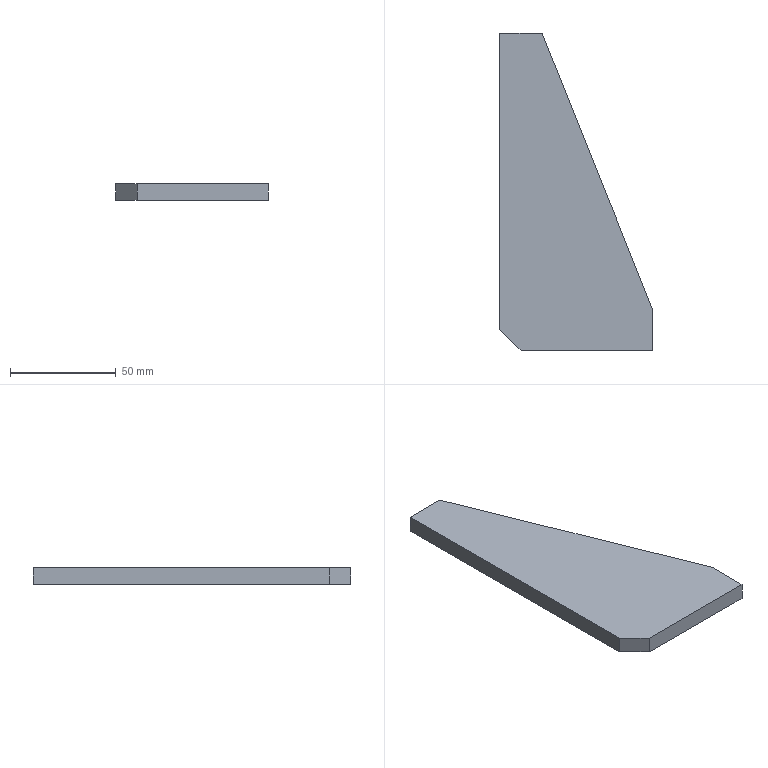Part | STEP file | 运输筋Plate 1 | 1 solid | 8 faces | box 72 x 150 x 8 mm | volume 58960 mm3 | plane 8
STEP:
#1=CARTESIAN_POINT('',(0.,0.,0.));
#2=DIRECTION('',(0.,0.,1.));
#3=DIRECTION('',(1.,0.,0.));
#4=AXIS2_PLACEMENT_3D('',#1,#2,#3);
#5=CARTESIAN_POINT('',(72.,0.,-4.));
#6=VERTEX_POINT('',#5);
#7=CARTESIAN_POINT('',(72.,20.,-4.));
#8=VERTEX_POINT('',#7);
#9=CARTESIAN_POINT('',(72.,0.,-4.));
#10=DIRECTION('',(0.,1.,0.));
#11=VECTOR('',#10,1.);
#12=LINE('',#9,#11);
#13=CARTESIAN_POINT('',(72.,0.,4.));
#14=DIRECTION('',(-1.,0.,0.));
#15=DIRECTION('',(0.,0.,1.));
#16=AXIS2_PLACEMENT_3D('',#13,#14,#15);
#17=PLANE('',#16);
#18=CARTESIAN_POINT('',(-8.,0.));
#19=DIRECTION('',(0.,1.));
#20=VECTOR('',#19,1.);
#21=LINE('',#18,#20);
#22=(GEOMETRIC_REPRESENTATION_CONTEXT(2)PARAMETRIC_REPRESENTATION_CONTEXT()REPRESENTATION_CONTEXT('',''));
#23=DEFINITIONAL_REPRESENTATION('',(#21),#22);
#24=PCURVE('',#17,#23);
#25=CARTESIAN_POINT('',(0.,0.,-4.));
#26=DIRECTION('',(0.,0.,1.));
#27=DIRECTION('',(1.,0.,0.));
#28=AXIS2_PLACEMENT_3D('',#25,#26,#27);
#29=PLANE('',#28);
#30=CARTESIAN_POINT('',(72.,0.));
#31=DIRECTION('',(0.,1.));
#32=VECTOR('',#31,1.);
#33=LINE('',#30,#32);
#34=(GEOMETRIC_REPRESENTATION_CONTEXT(2)PARAMETRIC_REPRESENTATION_CONTEXT()REPRESENTATION_CONTEXT('',''));
#35=DEFINITIONAL_REPRESENTATION('',(#33),#34);
#36=PCURVE('',#29,#35);
#37=SURFACE_CURVE('',#12,(#24,#36),.PCURVE_S1.);
#38=EDGE_CURVE('',#6,#8,#37,.T.);
#39=ORIENTED_EDGE('',*,*,#38,.T.);
#40=CARTESIAN_POINT('',(72.,20.,4.));
#41=VERTEX_POINT('',#40);
#42=CARTESIAN_POINT('',(72.,20.,4.));
#43=DIRECTION('',(0.,0.,-1.));
#44=VECTOR('',#43,1.);
#45=LINE('',#42,#44);
#46=CARTESIAN_POINT('',(0.,20.));
#47=DIRECTION('',(-1.,0.));
#48=VECTOR('',#47,1.);
#49=LINE('',#46,#48);
#50=(GEOMETRIC_REPRESENTATION_CONTEXT(2)PARAMETRIC_REPRESENTATION_CONTEXT()REPRESENTATION_CONTEXT('',''));
#51=DEFINITIONAL_REPRESENTATION('',(#49),#50);
#52=PCURVE('',#17,#51);
#53=CARTESIAN_POINT('',(72.,20.,4.));
#54=DIRECTION('',(-0.9285,-0.3714,0.));
#55=DIRECTION('',(0.3714,-0.9285,0.));
#56=AXIS2_PLACEMENT_3D('',#53,#54,#55);
#57=PLANE('',#56);
#58=CARTESIAN_POINT('',(0.,0.));
#59=DIRECTION('',(0.,-1.));
#60=VECTOR('',#59,1.);
#61=LINE('',#58,#60);
#62=(GEOMETRIC_REPRESENTATION_CONTEXT(2)PARAMETRIC_REPRESENTATION_CONTEXT()REPRESENTATION_CONTEXT('',''));
#63=DEFINITIONAL_REPRESENTATION('',(#61),#62);
#64=PCURVE('',#57,#63);
#65=SURFACE_CURVE('',#45,(#52,#64),.PCURVE_S1.);
#66=EDGE_CURVE('',#41,#8,#65,.T.);
#67=ORIENTED_EDGE('',*,*,#66,.F.);
#68=CARTESIAN_POINT('',(72.,0.,4.));
#69=VERTEX_POINT('',#68);
#70=CARTESIAN_POINT('',(72.,0.,4.));
#71=DIRECTION('',(0.,1.,0.));
#72=VECTOR('',#71,1.);
#73=LINE('',#70,#72);
#74=CARTESIAN_POINT('',(0.,0.));
#75=DIRECTION('',(0.,1.));
#76=VECTOR('',#75,1.);
#77=LINE('',#74,#76);
#78=(GEOMETRIC_REPRESENTATION_CONTEXT(2)PARAMETRIC_REPRESENTATION_CONTEXT()REPRESENTATION_CONTEXT('',''));
#79=DEFINITIONAL_REPRESENTATION('',(#77),#78);
#80=PCURVE('',#17,#79);
#81=CARTESIAN_POINT('',(0.,0.,4.));
#82=DIRECTION('',(0.,0.,1.));
#83=DIRECTION('',(1.,0.,0.));
#84=AXIS2_PLACEMENT_3D('',#81,#82,#83);
#85=PLANE('',#84);
#86=CARTESIAN_POINT('',(72.,0.));
#87=DIRECTION('',(0.,1.));
#88=VECTOR('',#87,1.);
#89=LINE('',#86,#88);
#90=(GEOMETRIC_REPRESENTATION_CONTEXT(2)PARAMETRIC_REPRESENTATION_CONTEXT()REPRESENTATION_CONTEXT('',''));
#91=DEFINITIONAL_REPRESENTATION('',(#89),#90);
#92=PCURVE('',#85,#91);
#93=SURFACE_CURVE('',#73,(#80,#92),.PCURVE_S1.);
#94=EDGE_CURVE('',#69,#41,#93,.T.);
#95=ORIENTED_EDGE('',*,*,#94,.F.);
#96=CARTESIAN_POINT('',(72.,0.,4.));
#97=DIRECTION('',(0.,0.,-1.));
#98=VECTOR('',#97,1.);
#99=LINE('',#96,#98);
#100=CARTESIAN_POINT('',(0.,0.));
#101=DIRECTION('',(-1.,0.));
#102=VECTOR('',#101,1.);
#103=LINE('',#100,#102);
#104=(GEOMETRIC_REPRESENTATION_CONTEXT(2)PARAMETRIC_REPRESENTATION_CONTEXT()REPRESENTATION_CONTEXT('',''));
#105=DEFINITIONAL_REPRESENTATION('',(#103),#104);
#106=PCURVE('',#17,#105);
#107=CARTESIAN_POINT('',(0.,0.,4.));
#108=DIRECTION('',(0.,1.,0.));
#109=DIRECTION('',(0.,0.,1.));
#110=AXIS2_PLACEMENT_3D('',#107,#108,#109);
#111=PLANE('',#110);
#112=CARTESIAN_POINT('',(0.,72.));
#113=DIRECTION('',(-1.,0.));
#114=VECTOR('',#113,1.);
#115=LINE('',#112,#114);
#116=(GEOMETRIC_REPRESENTATION_CONTEXT(2)PARAMETRIC_REPRESENTATION_CONTEXT()REPRESENTATION_CONTEXT('',''));
#117=DEFINITIONAL_REPRESENTATION('',(#115),#116);
#118=PCURVE('',#111,#117);
#119=SURFACE_CURVE('',#99,(#106,#118),.PCURVE_S1.);
#120=EDGE_CURVE('',#69,#6,#119,.T.);
#121=ORIENTED_EDGE('',*,*,#120,.T.);
#122=EDGE_LOOP('',(#39,#67,#95,#121));
#123=FACE_BOUND('',#122,.T.);
#124=ADVANCED_FACE('',(#123),#17,.F.);
#125=CARTESIAN_POINT('',(20.,150.,-4.));
#126=VERTEX_POINT('',#125);
#127=CARTESIAN_POINT('',(72.,20.,-4.));
#128=DIRECTION('',(-0.3714,0.9285,0.));
#129=VECTOR('',#128,1.);
#130=LINE('',#127,#129);
#131=CARTESIAN_POINT('',(0.,-8.));
#132=DIRECTION('',(-1.,0.));
#133=VECTOR('',#132,1.);
#134=LINE('',#131,#133);
#135=(GEOMETRIC_REPRESENTATION_CONTEXT(2)PARAMETRIC_REPRESENTATION_CONTEXT()REPRESENTATION_CONTEXT('',''));
#136=DEFINITIONAL_REPRESENTATION('',(#134),#135);
#137=PCURVE('',#57,#136);
#138=CARTESIAN_POINT('',(72.,20.));
#139=DIRECTION('',(-0.3714,0.9285));
#140=VECTOR('',#139,1.);
#141=LINE('',#138,#140);
#142=(GEOMETRIC_REPRESENTATION_CONTEXT(2)PARAMETRIC_REPRESENTATION_CONTEXT()REPRESENTATION_CONTEXT('',''));
#143=DEFINITIONAL_REPRESENTATION('',(#141),#142);
#144=PCURVE('',#29,#143);
#145=SURFACE_CURVE('',#130,(#137,#144),.PCURVE_S1.);
#146=EDGE_CURVE('',#8,#126,#145,.T.);
#147=ORIENTED_EDGE('',*,*,#146,.T.);
#148=CARTESIAN_POINT('',(20.,150.,4.));
#149=VERTEX_POINT('',#148);
#150=CARTESIAN_POINT('',(20.,150.,4.));
#151=DIRECTION('',(0.,0.,-1.));
#152=VECTOR('',#151,1.);
#153=LINE('',#150,#152);
#154=CARTESIAN_POINT('',(-140.014,0.));
#155=DIRECTION('',(0.,-1.));
#156=VECTOR('',#155,1.);
#157=LINE('',#154,#156);
#158=(GEOMETRIC_REPRESENTATION_CONTEXT(2)PARAMETRIC_REPRESENTATION_CONTEXT()REPRESENTATION_CONTEXT('',''));
#159=DEFINITIONAL_REPRESENTATION('',(#157),#158);
#160=PCURVE('',#57,#159);
#161=CARTESIAN_POINT('',(20.,150.,4.));
#162=DIRECTION('',(0.,-1.,0.));
#163=DIRECTION('',(0.,0.,-1.));
#164=AXIS2_PLACEMENT_3D('',#161,#162,#163);
#165=PLANE('',#164);
#166=CARTESIAN_POINT('',(0.,0.));
#167=DIRECTION('',(1.,0.));
#168=VECTOR('',#167,1.);
#169=LINE('',#166,#168);
#170=(GEOMETRIC_REPRESENTATION_CONTEXT(2)PARAMETRIC_REPRESENTATION_CONTEXT()REPRESENTATION_CONTEXT('',''));
#171=DEFINITIONAL_REPRESENTATION('',(#169),#170);
#172=PCURVE('',#165,#171);
#173=SURFACE_CURVE('',#153,(#160,#172),.PCURVE_S1.);
#174=EDGE_CURVE('',#149,#126,#173,.T.);
#175=ORIENTED_EDGE('',*,*,#174,.F.);
#176=CARTESIAN_POINT('',(72.,20.,4.));
#177=DIRECTION('',(-0.3714,0.9285,0.));
#178=VECTOR('',#177,1.);
#179=LINE('',#176,#178);
#180=CARTESIAN_POINT('',(0.,0.));
#181=DIRECTION('',(-1.,0.));
#182=VECTOR('',#181,1.);
#183=LINE('',#180,#182);
#184=(GEOMETRIC_REPRESENTATION_CONTEXT(2)PARAMETRIC_REPRESENTATION_CONTEXT()REPRESENTATION_CONTEXT('',''));
#185=DEFINITIONAL_REPRESENTATION('',(#183),#184);
#186=PCURVE('',#57,#185);
#187=CARTESIAN_POINT('',(72.,20.));
#188=DIRECTION('',(-0.3714,0.9285));
#189=VECTOR('',#188,1.);
#190=LINE('',#187,#189);
#191=(GEOMETRIC_REPRESENTATION_CONTEXT(2)PARAMETRIC_REPRESENTATION_CONTEXT()REPRESENTATION_CONTEXT('',''));
#192=DEFINITIONAL_REPRESENTATION('',(#190),#191);
#193=PCURVE('',#85,#192);
#194=SURFACE_CURVE('',#179,(#186,#193),.PCURVE_S1.);
#195=EDGE_CURVE('',#41,#149,#194,.T.);
#196=ORIENTED_EDGE('',*,*,#195,.F.);
#197=ORIENTED_EDGE('',*,*,#66,.T.);
#198=EDGE_LOOP('',(#147,#175,#196,#197));
#199=FACE_BOUND('',#198,.T.);
#200=ADVANCED_FACE('',(#199),#57,.F.);
#201=CARTESIAN_POINT('',(0.,150.,-4.));
#202=VERTEX_POINT('',#201);
#203=CARTESIAN_POINT('',(20.,150.,-4.));
#204=DIRECTION('',(-1.,0.,0.));
#205=VECTOR('',#204,1.);
#206=LINE('',#203,#205);
#207=CARTESIAN_POINT('',(8.,0.));
#208=DIRECTION('',(0.,-1.));
#209=VECTOR('',#208,1.);
#210=LINE('',#207,#209);
#211=(GEOMETRIC_REPRESENTATION_CONTEXT(2)PARAMETRIC_REPRESENTATION_CONTEXT()REPRESENTATION_CONTEXT('',''));
#212=DEFINITIONAL_REPRESENTATION('',(#210),#211);
#213=PCURVE('',#165,#212);
#214=CARTESIAN_POINT('',(20.,150.));
#215=DIRECTION('',(-1.,0.));
#216=VECTOR('',#215,1.);
#217=LINE('',#214,#216);
#218=(GEOMETRIC_REPRESENTATION_CONTEXT(2)PARAMETRIC_REPRESENTATION_CONTEXT()REPRESENTATION_CONTEXT('',''));
#219=DEFINITIONAL_REPRESENTATION('',(#217),#218);
#220=PCURVE('',#29,#219);
#221=SURFACE_CURVE('',#206,(#213,#220),.PCURVE_S1.);
#222=EDGE_CURVE('',#126,#202,#221,.T.);
#223=ORIENTED_EDGE('',*,*,#222,.T.);
#224=CARTESIAN_POINT('',(0.,150.,4.));
#225=VERTEX_POINT('',#224);
#226=CARTESIAN_POINT('',(0.,150.,4.));
#227=DIRECTION('',(0.,0.,-1.));
#228=VECTOR('',#227,1.);
#229=LINE('',#226,#228);
#230=CARTESIAN_POINT('',(0.,-20.));
#231=DIRECTION('',(1.,0.));
#232=VECTOR('',#231,1.);
#233=LINE('',#230,#232);
#234=(GEOMETRIC_REPRESENTATION_CONTEXT(2)PARAMETRIC_REPRESENTATION_CONTEXT()REPRESENTATION_CONTEXT('',''));
#235=DEFINITIONAL_REPRESENTATION('',(#233),#234);
#236=PCURVE('',#165,#235);
#237=CARTESIAN_POINT('',(0.,150.,4.));
#238=DIRECTION('',(1.,0.,0.));
#239=DIRECTION('',(0.,1.,0.));
#240=AXIS2_PLACEMENT_3D('',#237,#238,#239);
#241=PLANE('',#240);
#242=CARTESIAN_POINT('',(0.,0.));
#243=DIRECTION('',(0.,-1.));
#244=VECTOR('',#243,1.);
#245=LINE('',#242,#244);
#246=(GEOMETRIC_REPRESENTATION_CONTEXT(2)PARAMETRIC_REPRESENTATION_CONTEXT()REPRESENTATION_CONTEXT('',''));
#247=DEFINITIONAL_REPRESENTATION('',(#245),#246);
#248=PCURVE('',#241,#247);
#249=SURFACE_CURVE('',#229,(#236,#248),.PCURVE_S1.);
#250=EDGE_CURVE('',#225,#202,#249,.T.);
#251=ORIENTED_EDGE('',*,*,#250,.F.);
#252=CARTESIAN_POINT('',(20.,150.,4.));
#253=DIRECTION('',(-1.,0.,0.));
#254=VECTOR('',#253,1.);
#255=LINE('',#252,#254);
#256=CARTESIAN_POINT('',(0.,0.));
#257=DIRECTION('',(0.,-1.));
#258=VECTOR('',#257,1.);
#259=LINE('',#256,#258);
#260=(GEOMETRIC_REPRESENTATION_CONTEXT(2)PARAMETRIC_REPRESENTATION_CONTEXT()REPRESENTATION_CONTEXT('',''));
#261=DEFINITIONAL_REPRESENTATION('',(#259),#260);
#262=PCURVE('',#165,#261);
#263=CARTESIAN_POINT('',(20.,150.));
#264=DIRECTION('',(-1.,0.));
#265=VECTOR('',#264,1.);
#266=LINE('',#263,#265);
#267=(GEOMETRIC_REPRESENTATION_CONTEXT(2)PARAMETRIC_REPRESENTATION_CONTEXT()REPRESENTATION_CONTEXT('',''));
#268=DEFINITIONAL_REPRESENTATION('',(#266),#267);
#269=PCURVE('',#85,#268);
#270=SURFACE_CURVE('',#255,(#262,#269),.PCURVE_S1.);
#271=EDGE_CURVE('',#149,#225,#270,.T.);
#272=ORIENTED_EDGE('',*,*,#271,.F.);
#273=ORIENTED_EDGE('',*,*,#174,.T.);
#274=EDGE_LOOP('',(#223,#251,#272,#273));
#275=FACE_BOUND('',#274,.T.);
#276=ADVANCED_FACE('',(#275),#165,.F.);
#277=CARTESIAN_POINT('',(0.,10.,-4.));
#278=VERTEX_POINT('',#277);
#279=CARTESIAN_POINT('',(0.,150.,-4.));
#280=DIRECTION('',(0.,-1.,0.));
#281=VECTOR('',#280,1.);
#282=LINE('',#279,#281);
#283=CARTESIAN_POINT('',(0.,-8.));
#284=DIRECTION('',(-1.,0.));
#285=VECTOR('',#284,1.);
#286=LINE('',#283,#285);
#287=(GEOMETRIC_REPRESENTATION_CONTEXT(2)PARAMETRIC_REPRESENTATION_CONTEXT()REPRESENTATION_CONTEXT('',''));
#288=DEFINITIONAL_REPRESENTATION('',(#286),#287);
#289=PCURVE('',#241,#288);
#290=CARTESIAN_POINT('',(0.,150.));
#291=DIRECTION('',(0.,-1.));
#292=VECTOR('',#291,1.);
#293=LINE('',#290,#292);
#294=(GEOMETRIC_REPRESENTATION_CONTEXT(2)PARAMETRIC_REPRESENTATION_CONTEXT()REPRESENTATION_CONTEXT('',''));
#295=DEFINITIONAL_REPRESENTATION('',(#293),#294);
#296=PCURVE('',#29,#295);
#297=SURFACE_CURVE('',#282,(#289,#296),.PCURVE_S1.);
#298=EDGE_CURVE('',#202,#278,#297,.T.);
#299=ORIENTED_EDGE('',*,*,#298,.T.);
#300=CARTESIAN_POINT('',(0.,10.,4.));
#301=VERTEX_POINT('',#300);
#302=CARTESIAN_POINT('',(0.,10.,4.));
#303=DIRECTION('',(0.,0.,1.));
#304=VECTOR('',#303,1.);
#305=LINE('',#302,#304);
#306=CARTESIAN_POINT('',(-140.,0.));
#307=DIRECTION('',(0.,1.));
#308=VECTOR('',#307,1.);
#309=LINE('',#306,#308);
#310=(GEOMETRIC_REPRESENTATION_CONTEXT(2)PARAMETRIC_REPRESENTATION_CONTEXT()REPRESENTATION_CONTEXT('',''));
#311=DEFINITIONAL_REPRESENTATION('',(#309),#310);
#312=PCURVE('',#241,#311);
#313=CARTESIAN_POINT('',(10.,0.,4.));
#314=DIRECTION('',(0.7071,0.7071,0.));
#315=DIRECTION('',(0.,0.,-1.));
#316=AXIS2_PLACEMENT_3D('',#313,#314,#315);
#317=PLANE('',#316);
#318=CARTESIAN_POINT('',(0.,14.142));
#319=DIRECTION('',(-1.,0.));
#320=VECTOR('',#319,1.);
#321=LINE('',#318,#320);
#322=(GEOMETRIC_REPRESENTATION_CONTEXT(2)PARAMETRIC_REPRESENTATION_CONTEXT()REPRESENTATION_CONTEXT('',''));
#323=DEFINITIONAL_REPRESENTATION('',(#321),#322);
#324=PCURVE('',#317,#323);
#325=SURFACE_CURVE('',#305,(#312,#324),.PCURVE_S1.);
#326=EDGE_CURVE('',#278,#301,#325,.T.);
#327=ORIENTED_EDGE('',*,*,#326,.T.);
#328=CARTESIAN_POINT('',(0.,150.,4.));
#329=DIRECTION('',(0.,-1.,0.));
#330=VECTOR('',#329,1.);
#331=LINE('',#328,#330);
#332=CARTESIAN_POINT('',(0.,0.));
#333=DIRECTION('',(-1.,0.));
#334=VECTOR('',#333,1.);
#335=LINE('',#332,#334);
#336=(GEOMETRIC_REPRESENTATION_CONTEXT(2)PARAMETRIC_REPRESENTATION_CONTEXT()REPRESENTATION_CONTEXT('',''));
#337=DEFINITIONAL_REPRESENTATION('',(#335),#336);
#338=PCURVE('',#241,#337);
#339=CARTESIAN_POINT('',(0.,150.));
#340=DIRECTION('',(0.,-1.));
#341=VECTOR('',#340,1.);
#342=LINE('',#339,#341);
#343=(GEOMETRIC_REPRESENTATION_CONTEXT(2)PARAMETRIC_REPRESENTATION_CONTEXT()REPRESENTATION_CONTEXT('',''));
#344=DEFINITIONAL_REPRESENTATION('',(#342),#343);
#345=PCURVE('',#85,#344);
#346=SURFACE_CURVE('',#331,(#338,#345),.PCURVE_S1.);
#347=EDGE_CURVE('',#225,#301,#346,.T.);
#348=ORIENTED_EDGE('',*,*,#347,.F.);
#349=ORIENTED_EDGE('',*,*,#250,.T.);
#350=EDGE_LOOP('',(#299,#327,#348,#349));
#351=FACE_BOUND('',#350,.T.);
#352=ADVANCED_FACE('',(#351),#241,.F.);
#353=CARTESIAN_POINT('',(10.,0.,4.));
#354=VERTEX_POINT('',#353);
#355=CARTESIAN_POINT('',(0.,0.,4.));
#356=DIRECTION('',(1.,0.,0.));
#357=VECTOR('',#356,1.);
#358=LINE('',#355,#357);
#359=CARTESIAN_POINT('',(0.,0.));
#360=DIRECTION('',(0.,1.));
#361=VECTOR('',#360,1.);
#362=LINE('',#359,#361);
#363=(GEOMETRIC_REPRESENTATION_CONTEXT(2)PARAMETRIC_REPRESENTATION_CONTEXT()REPRESENTATION_CONTEXT('',''));
#364=DEFINITIONAL_REPRESENTATION('',(#362),#363);
#365=PCURVE('',#111,#364);
#366=CARTESIAN_POINT('',(0.,0.));
#367=DIRECTION('',(1.,0.));
#368=VECTOR('',#367,1.);
#369=LINE('',#366,#368);
#370=(GEOMETRIC_REPRESENTATION_CONTEXT(2)PARAMETRIC_REPRESENTATION_CONTEXT()REPRESENTATION_CONTEXT('',''));
#371=DEFINITIONAL_REPRESENTATION('',(#369),#370);
#372=PCURVE('',#85,#371);
#373=SURFACE_CURVE('',#358,(#365,#372),.PCURVE_S1.);
#374=EDGE_CURVE('',#354,#69,#373,.T.);
#375=ORIENTED_EDGE('',*,*,#374,.F.);
#376=CARTESIAN_POINT('',(10.,0.,-4.));
#377=VERTEX_POINT('',#376);
#378=CARTESIAN_POINT('',(10.,0.,4.));
#379=DIRECTION('',(0.,0.,-1.));
#380=VECTOR('',#379,1.);
#381=LINE('',#378,#380);
#382=CARTESIAN_POINT('',(0.,10.));
#383=DIRECTION('',(-1.,0.));
#384=VECTOR('',#383,1.);
#385=LINE('',#382,#384);
#386=(GEOMETRIC_REPRESENTATION_CONTEXT(2)PARAMETRIC_REPRESENTATION_CONTEXT()REPRESENTATION_CONTEXT('',''));
#387=DEFINITIONAL_REPRESENTATION('',(#385),#386);
#388=PCURVE('',#111,#387);
#389=CARTESIAN_POINT('',(0.,0.));
#390=DIRECTION('',(1.,0.));
#391=VECTOR('',#390,1.);
#392=LINE('',#389,#391);
#393=(GEOMETRIC_REPRESENTATION_CONTEXT(2)PARAMETRIC_REPRESENTATION_CONTEXT()REPRESENTATION_CONTEXT('',''));
#394=DEFINITIONAL_REPRESENTATION('',(#392),#393);
#395=PCURVE('',#317,#394);
#396=SURFACE_CURVE('',#381,(#388,#395),.PCURVE_S1.);
#397=EDGE_CURVE('',#354,#377,#396,.T.);
#398=ORIENTED_EDGE('',*,*,#397,.T.);
#399=CARTESIAN_POINT('',(0.,0.,-4.));
#400=DIRECTION('',(1.,0.,0.));
#401=VECTOR('',#400,1.);
#402=LINE('',#399,#401);
#403=CARTESIAN_POINT('',(-8.,0.));
#404=DIRECTION('',(0.,1.));
#405=VECTOR('',#404,1.);
#406=LINE('',#403,#405);
#407=(GEOMETRIC_REPRESENTATION_CONTEXT(2)PARAMETRIC_REPRESENTATION_CONTEXT()REPRESENTATION_CONTEXT('',''));
#408=DEFINITIONAL_REPRESENTATION('',(#406),#407);
#409=PCURVE('',#111,#408);
#410=CARTESIAN_POINT('',(0.,0.));
#411=DIRECTION('',(1.,0.));
#412=VECTOR('',#411,1.);
#413=LINE('',#410,#412);
#414=(GEOMETRIC_REPRESENTATION_CONTEXT(2)PARAMETRIC_REPRESENTATION_CONTEXT()REPRESENTATION_CONTEXT('',''));
#415=DEFINITIONAL_REPRESENTATION('',(#413),#414);
#416=PCURVE('',#29,#415);
#417=SURFACE_CURVE('',#402,(#409,#416),.PCURVE_S1.);
#418=EDGE_CURVE('',#377,#6,#417,.T.);
#419=ORIENTED_EDGE('',*,*,#418,.T.);
#420=ORIENTED_EDGE('',*,*,#120,.F.);
#421=EDGE_LOOP('',(#375,#398,#419,#420));
#422=FACE_BOUND('',#421,.T.);
#423=ADVANCED_FACE('',(#422),#111,.F.);
#424=ORIENTED_EDGE('',*,*,#347,.T.);
#425=CARTESIAN_POINT('',(5.,5.,4.));
#426=DIRECTION('',(0.7071,-0.7071,0.));
#427=VECTOR('',#426,1.);
#428=LINE('',#425,#427);
#429=CARTESIAN_POINT('',(5.,5.));
#430=DIRECTION('',(0.7071,-0.7071));
#431=VECTOR('',#430,1.);
#432=LINE('',#429,#431);
#433=(GEOMETRIC_REPRESENTATION_CONTEXT(2)PARAMETRIC_REPRESENTATION_CONTEXT()REPRESENTATION_CONTEXT('',''));
#434=DEFINITIONAL_REPRESENTATION('',(#432),#433);
#435=PCURVE('',#85,#434);
#436=CARTESIAN_POINT('',(0.,7.071));
#437=DIRECTION('',(0.,-1.));
#438=VECTOR('',#437,1.);
#439=LINE('',#436,#438);
#440=(GEOMETRIC_REPRESENTATION_CONTEXT(2)PARAMETRIC_REPRESENTATION_CONTEXT()REPRESENTATION_CONTEXT('',''));
#441=DEFINITIONAL_REPRESENTATION('',(#439),#440);
#442=PCURVE('',#317,#441);
#443=SURFACE_CURVE('',#428,(#435,#442),.PCURVE_S1.);
#444=EDGE_CURVE('',#301,#354,#443,.T.);
#445=ORIENTED_EDGE('',*,*,#444,.T.);
#446=ORIENTED_EDGE('',*,*,#374,.T.);
#447=ORIENTED_EDGE('',*,*,#94,.T.);
#448=ORIENTED_EDGE('',*,*,#195,.T.);
#449=ORIENTED_EDGE('',*,*,#271,.T.);
#450=EDGE_LOOP('',(#424,#445,#446,#447,#448,#449));
#451=FACE_BOUND('',#450,.T.);
#452=ADVANCED_FACE('',(#451),#85,.T.);
#453=ORIENTED_EDGE('',*,*,#418,.F.);
#454=CARTESIAN_POINT('',(10.,0.,-4.));
#455=DIRECTION('',(-0.7071,0.7071,0.));
#456=VECTOR('',#455,1.);
#457=LINE('',#454,#456);
#458=CARTESIAN_POINT('',(10.,0.));
#459=DIRECTION('',(-0.7071,0.7071));
#460=VECTOR('',#459,1.);
#461=LINE('',#458,#460);
#462=(GEOMETRIC_REPRESENTATION_CONTEXT(2)PARAMETRIC_REPRESENTATION_CONTEXT()REPRESENTATION_CONTEXT('',''));
#463=DEFINITIONAL_REPRESENTATION('',(#461),#462);
#464=PCURVE('',#29,#463);
#465=CARTESIAN_POINT('',(8.,0.));
#466=DIRECTION('',(0.,1.));
#467=VECTOR('',#466,1.);
#468=LINE('',#465,#467);
#469=(GEOMETRIC_REPRESENTATION_CONTEXT(2)PARAMETRIC_REPRESENTATION_CONTEXT()REPRESENTATION_CONTEXT('',''));
#470=DEFINITIONAL_REPRESENTATION('',(#468),#469);
#471=PCURVE('',#317,#470);
#472=SURFACE_CURVE('',#457,(#464,#471),.PCURVE_S1.);
#473=EDGE_CURVE('',#377,#278,#472,.T.);
#474=ORIENTED_EDGE('',*,*,#473,.T.);
#475=ORIENTED_EDGE('',*,*,#298,.F.);
#476=ORIENTED_EDGE('',*,*,#222,.F.);
#477=ORIENTED_EDGE('',*,*,#146,.F.);
#478=ORIENTED_EDGE('',*,*,#38,.F.);
#479=EDGE_LOOP('',(#453,#474,#475,#476,#477,#478));
#480=FACE_BOUND('',#479,.T.);
#481=ADVANCED_FACE('',(#480),#29,.F.);
#482=ORIENTED_EDGE('',*,*,#444,.F.);
#483=ORIENTED_EDGE('',*,*,#326,.F.);
#484=ORIENTED_EDGE('',*,*,#473,.F.);
#485=ORIENTED_EDGE('',*,*,#397,.F.);
#486=EDGE_LOOP('',(#482,#483,#484,#485));
#487=FACE_BOUND('',#486,.T.);
#488=ADVANCED_FACE('',(#487),#317,.F.);
#489=CLOSED_SHELL('',(#124,#200,#276,#352,#423,#452,#481,#488));
#490=MANIFOLD_SOLID_BREP('',#489);
#491=(LENGTH_UNIT()NAMED_UNIT(*)SI_UNIT(.MILLI.,.METRE.));
#492=UNCERTAINTY_MEASURE_WITH_UNIT(LENGTH_MEASURE(0.0000001),#491,'','');
#493=(NAMED_UNIT(*)PLANE_ANGLE_UNIT()SI_UNIT($,.RADIAN.));
#494=(NAMED_UNIT(*)SI_UNIT($,.STERADIAN.)SOLID_ANGLE_UNIT());
#495=(GEOMETRIC_REPRESENTATION_CONTEXT(3)GLOBAL_UNCERTAINTY_ASSIGNED_CONTEXT((#492))GLOBAL_UNIT_ASSIGNED_CONTEXT((#491,#493,#494))REPRESENTATION_CONTEXT('',''));
#496=ADVANCED_BREP_SHAPE_REPRESENTATION('',(#4,#490),#495);